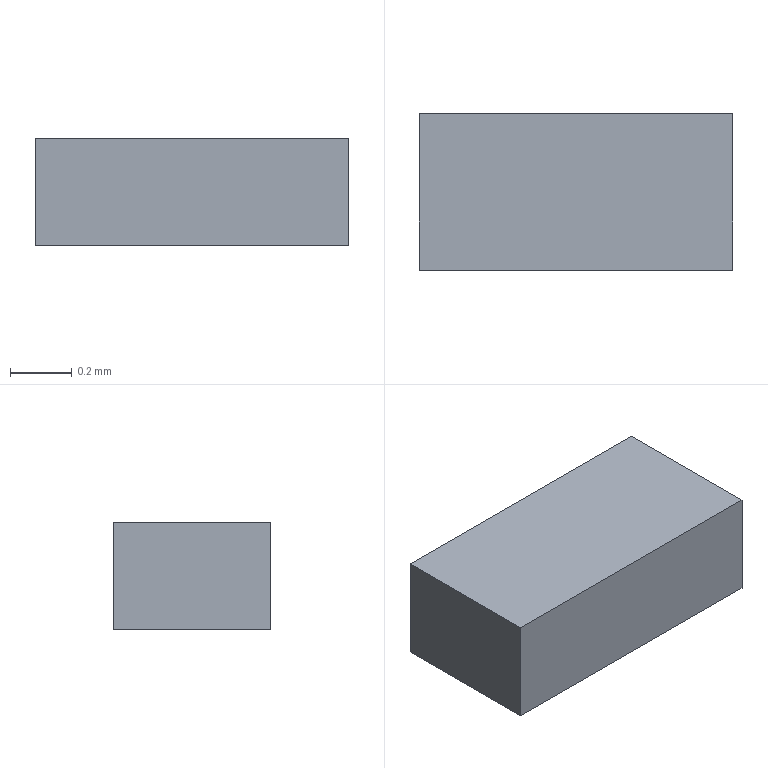Part | Creo | 1 solid | 6 faces | box 1.016 x 0.508 x 0.35 mm | volume 0.1806 mm3 | plane 6
STEP:
#1=CARTESIAN_POINT('',(0.,0.,0.));
#2=DIRECTION('',(0.,0.,1.));
#3=DIRECTION('',(1.,0.,0.));
#4=AXIS2_PLACEMENT_3D('',#1,#2,#3);
#5=CARTESIAN_POINT('',(-0.508,0.254,0.));
#6=VERTEX_POINT('',#5);
#7=CARTESIAN_POINT('',(-0.508,-0.254,0.));
#8=VERTEX_POINT('',#7);
#9=CARTESIAN_POINT('',(-0.508,0.254,0.));
#10=DIRECTION('',(0.,-1.,0.));
#11=VECTOR('',#10,0.508);
#12=LINE('',#9,#11);
#13=EDGE_CURVE('',#6,#8,#12,.T.);
#14=ORIENTED_EDGE('',*,*,#13,.T.);
#15=CARTESIAN_POINT('',(0.508,-0.254,0.));
#16=VERTEX_POINT('',#15);
#17=CARTESIAN_POINT('',(-0.508,-0.254,0.));
#18=DIRECTION('',(1.,0.,0.));
#19=VECTOR('',#18,1.016);
#20=LINE('',#17,#19);
#21=EDGE_CURVE('',#8,#16,#20,.T.);
#22=ORIENTED_EDGE('',*,*,#21,.T.);
#23=CARTESIAN_POINT('',(0.508,0.254,0.));
#24=VERTEX_POINT('',#23);
#25=CARTESIAN_POINT('',(0.508,-0.254,0.));
#26=DIRECTION('',(0.,1.,0.));
#27=VECTOR('',#26,0.508);
#28=LINE('',#25,#27);
#29=EDGE_CURVE('',#16,#24,#28,.T.);
#30=ORIENTED_EDGE('',*,*,#29,.T.);
#31=CARTESIAN_POINT('',(0.508,0.254,0.));
#32=DIRECTION('',(-1.,0.,0.));
#33=VECTOR('',#32,1.016);
#34=LINE('',#31,#33);
#35=EDGE_CURVE('',#24,#6,#34,.T.);
#36=ORIENTED_EDGE('',*,*,#35,.T.);
#37=EDGE_LOOP('',(#14,#22,#30,#36));
#38=FACE_OUTER_BOUND('',#37,.F.);
#39=CARTESIAN_POINT('',(0.,0.,0.));
#40=DIRECTION('',(0.,0.,1.));
#41=DIRECTION('',(1.,0.,0.));
#42=AXIS2_PLACEMENT_3D('',#39,#40,#41);
#43=PLANE('',#42);
#44=ADVANCED_FACE('',(#38),#43,.F.);
#45=ORIENTED_EDGE('',*,*,#13,.F.);
#46=CARTESIAN_POINT('',(-0.508,0.254,0.35));
#47=VERTEX_POINT('',#46);
#48=CARTESIAN_POINT('',(-0.508,0.254,0.));
#49=DIRECTION('',(0.,0.,1.));
#50=VECTOR('',#49,0.35);
#51=LINE('',#48,#50);
#52=EDGE_CURVE('',#6,#47,#51,.T.);
#53=ORIENTED_EDGE('',*,*,#52,.T.);
#54=CARTESIAN_POINT('',(-0.508,-0.254,0.35));
#55=VERTEX_POINT('',#54);
#56=CARTESIAN_POINT('',(-0.508,0.254,0.35));
#57=DIRECTION('',(0.,-1.,0.));
#58=VECTOR('',#57,0.508);
#59=LINE('',#56,#58);
#60=EDGE_CURVE('',#47,#55,#59,.T.);
#61=ORIENTED_EDGE('',*,*,#60,.T.);
#62=CARTESIAN_POINT('',(-0.508,-0.254,0.));
#63=DIRECTION('',(0.,0.,1.));
#64=VECTOR('',#63,0.35);
#65=LINE('',#62,#64);
#66=EDGE_CURVE('',#8,#55,#65,.T.);
#67=ORIENTED_EDGE('',*,*,#66,.F.);
#68=EDGE_LOOP('',(#45,#53,#61,#67));
#69=FACE_OUTER_BOUND('',#68,.F.);
#70=CARTESIAN_POINT('',(-0.508,0.254,0.));
#71=DIRECTION('',(-1.,0.,0.));
#72=DIRECTION('',(0.,-1.,0.));
#73=AXIS2_PLACEMENT_3D('',#70,#71,#72);
#74=PLANE('',#73);
#75=ADVANCED_FACE('',(#69),#74,.T.);
#76=ORIENTED_EDGE('',*,*,#35,.F.);
#77=CARTESIAN_POINT('',(0.508,0.254,0.35));
#78=VERTEX_POINT('',#77);
#79=CARTESIAN_POINT('',(0.508,0.254,0.));
#80=DIRECTION('',(0.,0.,1.));
#81=VECTOR('',#80,0.35);
#82=LINE('',#79,#81);
#83=EDGE_CURVE('',#24,#78,#82,.T.);
#84=ORIENTED_EDGE('',*,*,#83,.T.);
#85=CARTESIAN_POINT('',(0.508,0.254,0.35));
#86=DIRECTION('',(-1.,0.,0.));
#87=VECTOR('',#86,1.016);
#88=LINE('',#85,#87);
#89=EDGE_CURVE('',#78,#47,#88,.T.);
#90=ORIENTED_EDGE('',*,*,#89,.T.);
#91=ORIENTED_EDGE('',*,*,#52,.F.);
#92=EDGE_LOOP('',(#76,#84,#90,#91));
#93=FACE_OUTER_BOUND('',#92,.F.);
#94=CARTESIAN_POINT('',(0.508,0.254,0.));
#95=DIRECTION('',(0.,1.,0.));
#96=DIRECTION('',(-1.,0.,0.));
#97=AXIS2_PLACEMENT_3D('',#94,#95,#96);
#98=PLANE('',#97);
#99=ADVANCED_FACE('',(#93),#98,.T.);
#100=ORIENTED_EDGE('',*,*,#29,.F.);
#101=CARTESIAN_POINT('',(0.508,-0.254,0.35));
#102=VERTEX_POINT('',#101);
#103=CARTESIAN_POINT('',(0.508,-0.254,0.));
#104=DIRECTION('',(0.,0.,1.));
#105=VECTOR('',#104,0.35);
#106=LINE('',#103,#105);
#107=EDGE_CURVE('',#16,#102,#106,.T.);
#108=ORIENTED_EDGE('',*,*,#107,.T.);
#109=CARTESIAN_POINT('',(0.508,-0.254,0.35));
#110=DIRECTION('',(0.,1.,0.));
#111=VECTOR('',#110,0.508);
#112=LINE('',#109,#111);
#113=EDGE_CURVE('',#102,#78,#112,.T.);
#114=ORIENTED_EDGE('',*,*,#113,.T.);
#115=ORIENTED_EDGE('',*,*,#83,.F.);
#116=EDGE_LOOP('',(#100,#108,#114,#115));
#117=FACE_OUTER_BOUND('',#116,.F.);
#118=CARTESIAN_POINT('',(0.508,-0.254,0.));
#119=DIRECTION('',(1.,0.,0.));
#120=DIRECTION('',(0.,1.,0.));
#121=AXIS2_PLACEMENT_3D('',#118,#119,#120);
#122=PLANE('',#121);
#123=ADVANCED_FACE('',(#117),#122,.T.);
#124=ORIENTED_EDGE('',*,*,#21,.F.);
#125=ORIENTED_EDGE('',*,*,#66,.T.);
#126=CARTESIAN_POINT('',(-0.508,-0.254,0.35));
#127=DIRECTION('',(1.,0.,0.));
#128=VECTOR('',#127,1.016);
#129=LINE('',#126,#128);
#130=EDGE_CURVE('',#55,#102,#129,.T.);
#131=ORIENTED_EDGE('',*,*,#130,.T.);
#132=ORIENTED_EDGE('',*,*,#107,.F.);
#133=EDGE_LOOP('',(#124,#125,#131,#132));
#134=FACE_OUTER_BOUND('',#133,.F.);
#135=CARTESIAN_POINT('',(-0.508,-0.254,0.));
#136=DIRECTION('',(0.,-1.,0.));
#137=DIRECTION('',(1.,0.,0.));
#138=AXIS2_PLACEMENT_3D('',#135,#136,#137);
#139=PLANE('',#138);
#140=ADVANCED_FACE('',(#134),#139,.T.);
#141=ORIENTED_EDGE('',*,*,#60,.F.);
#142=ORIENTED_EDGE('',*,*,#89,.F.);
#143=ORIENTED_EDGE('',*,*,#113,.F.);
#144=ORIENTED_EDGE('',*,*,#130,.F.);
#145=EDGE_LOOP('',(#141,#142,#143,#144));
#146=FACE_OUTER_BOUND('',#145,.F.);
#147=CARTESIAN_POINT('',(0.,0.,0.35));
#148=DIRECTION('',(0.,0.,1.));
#149=DIRECTION('',(1.,0.,0.));
#150=AXIS2_PLACEMENT_3D('',#147,#148,#149);
#151=PLANE('',#150);
#152=ADVANCED_FACE('',(#146),#151,.T.);
#153=CLOSED_SHELL('',(#44,#75,#99,#123,#140,#152));
#154=MANIFOLD_SOLID_BREP('',#153);
#155=(LENGTH_UNIT()NAMED_UNIT(*)SI_UNIT(.MILLI.,.METRE.));
#156=UNCERTAINTY_MEASURE_WITH_UNIT(LENGTH_MEASURE(0.0001189),#155,'','');
#157=(NAMED_UNIT(*)PLANE_ANGLE_UNIT()SI_UNIT($,.RADIAN.));
#158=PLANE_ANGLE_MEASURE_WITH_UNIT(PLANE_ANGLE_MEASURE(0.01745),#157);
#159=(CONVERSION_BASED_UNIT('DEGREE',#158)NAMED_UNIT(*)PLANE_ANGLE_UNIT());
#160=(NAMED_UNIT(*)SI_UNIT($,.STERADIAN.)SOLID_ANGLE_UNIT());
#161=(GEOMETRIC_REPRESENTATION_CONTEXT(3)GLOBAL_UNCERTAINTY_ASSIGNED_CONTEXT((#156))GLOBAL_UNIT_ASSIGNED_CONTEXT((#155,#159,#160))REPRESENTATION_CONTEXT('',''));
#162=ADVANCED_BREP_SHAPE_REPRESENTATION('',(#4,#154),#161);